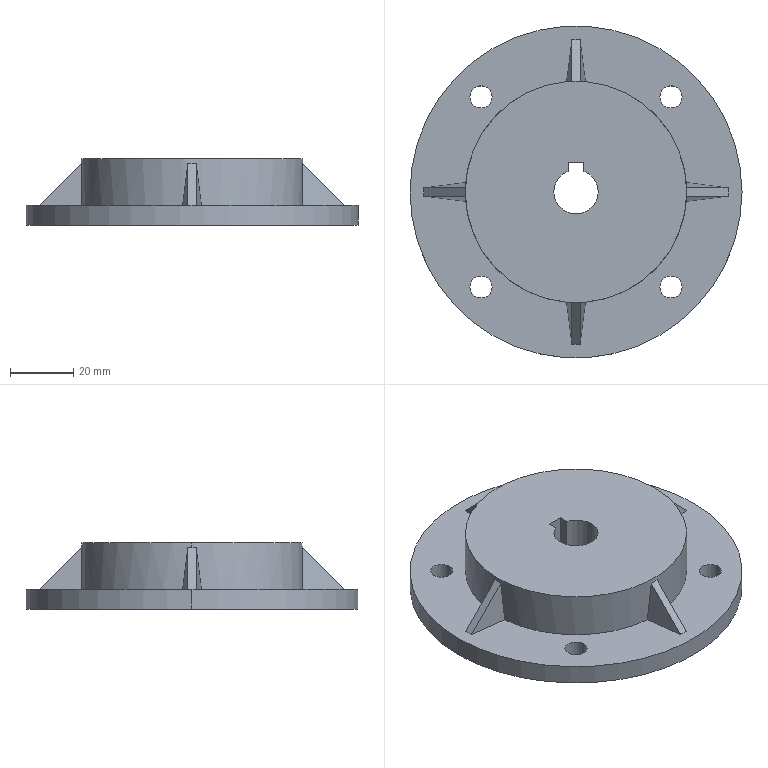Part | STEP file | Input motor flange_063_P71B14.step | 1 solid | 236 faces | box 105 x 105 x 21 mm | volume 72142 mm3 | plane 154 | cylinder 77 | cone 5 | commonest cylinder face diameters 9.1 x16 75.25 x13 99.75 x13 10.55 x12 7 x8 70 x4